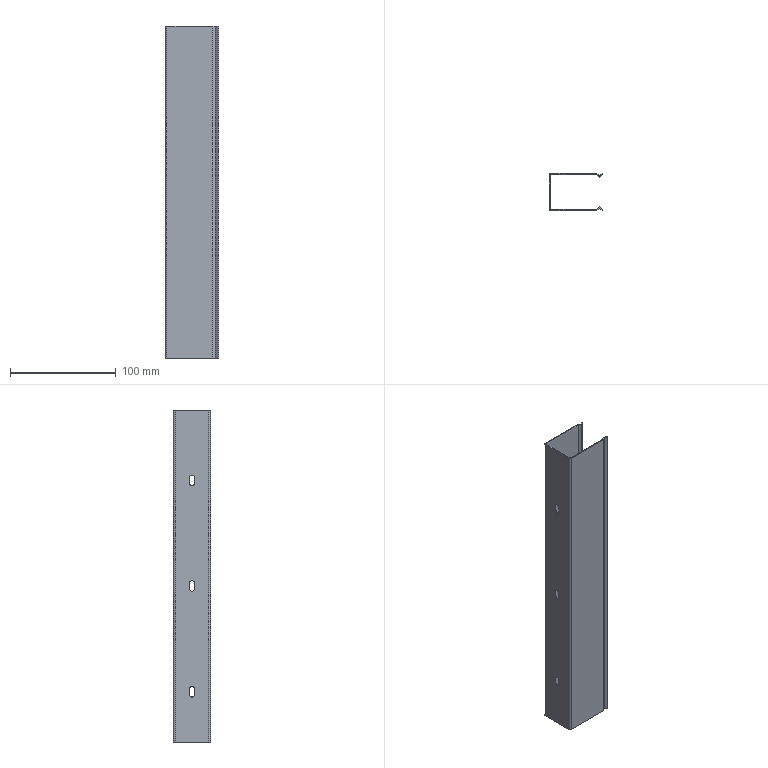Part | STEP file | 35 Cable Tray_314 | 1 solid | 37 faces | box 50.625 x 35 x 314 mm | volume 42522 mm3 | plane 24 | cylinder 13 | commonest cylinder face diameters 5 x9 1 x2 3 x2